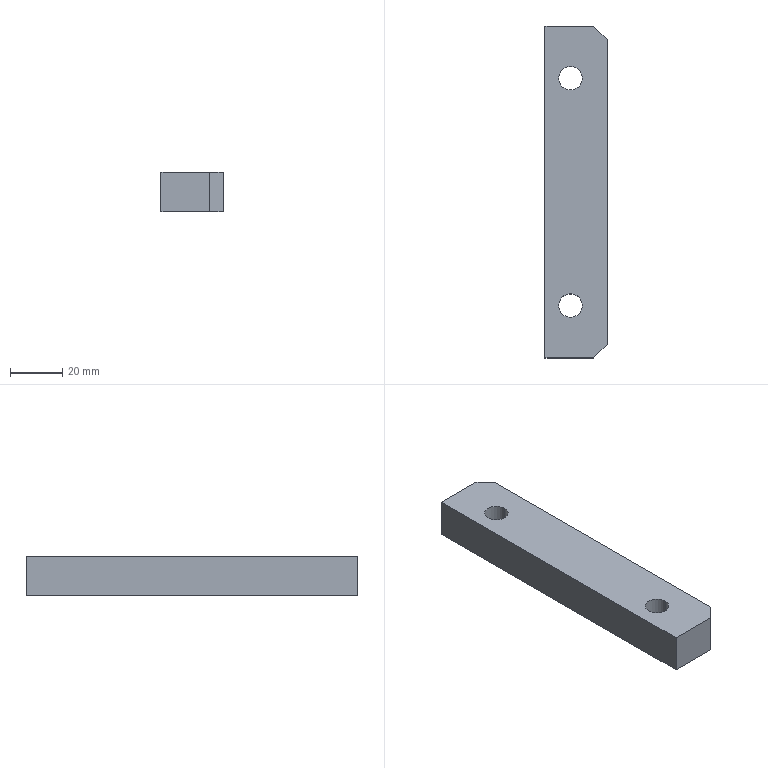Part | 1 solid | 26 faces | box 23.738 x 127 x 15 mm | volume 40590 mm3 | cylinder 12 | plane 10 | cone 4 | commonest cylinder face diameters 8 x4 9 x4 14 x4